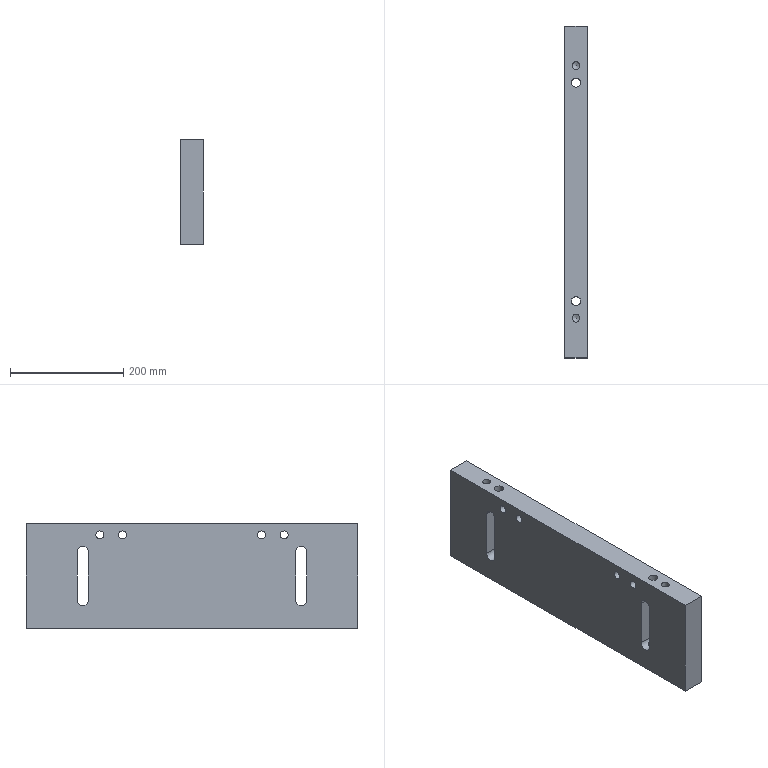Part | STEP file | 1 solid | 32 faces | box 40 x 585 x 185 mm | volume 4078797 mm3 | cylinder 17 | plane 10 | cone 5 | commonest cylinder face diameters 14 x9 16 x4 20 x4
STEP:
#1=CARTESIAN_POINT('',(-360.,-182.5,-242.));
#2=VERTEX_POINT('',#1);
#3=CARTESIAN_POINT('',(-360.,-202.5,-242.));
#4=VERTEX_POINT('',#3);
#5=CARTESIAN_POINT('',(-360.,-192.5,-242.));
#6=DIRECTION('',(-1.,0.,0.));
#7=DIRECTION('',(0.,0.,1.));
#8=AXIS2_PLACEMENT_3D('',#5,#6,#7);
#9=CIRCLE('',#8,10.);
#10=EDGE_CURVE('',#2,#4,#9,.T.);
#11=ORIENTED_EDGE('',*,*,#10,.F.);
#12=CARTESIAN_POINT('',(-360.,-182.5,-157.));
#13=VERTEX_POINT('',#12);
#14=CARTESIAN_POINT('',(-360.,-182.5,-292.));
#15=DIRECTION('',(0.,0.,1.));
#16=VECTOR('',#15,1.);
#17=LINE('',#14,#16);
#18=EDGE_CURVE('',#2,#13,#17,.T.);
#19=ORIENTED_EDGE('',*,*,#18,.T.);
#20=CARTESIAN_POINT('',(-360.,-202.5,-157.));
#21=VERTEX_POINT('',#20);
#22=CARTESIAN_POINT('',(-360.,-192.5,-157.));
#23=DIRECTION('',(-1.,0.,0.));
#24=DIRECTION('',(0.,0.,1.));
#25=AXIS2_PLACEMENT_3D('',#22,#23,#24);
#26=CIRCLE('',#25,10.);
#27=EDGE_CURVE('',#21,#13,#26,.T.);
#28=ORIENTED_EDGE('',*,*,#27,.F.);
#29=CARTESIAN_POINT('',(-360.,-202.5,-107.));
#30=DIRECTION('',(0.,0.,1.));
#31=VECTOR('',#30,1.);
#32=LINE('',#29,#31);
#33=EDGE_CURVE('',#4,#21,#32,.T.);
#34=ORIENTED_EDGE('',*,*,#33,.F.);
#35=EDGE_LOOP('',(#11,#19,#28,#34));
#36=FACE_BOUND('',#35,.T.);
#37=CARTESIAN_POINT('',(-360.,-292.5,-292.));
#38=VERTEX_POINT('',#37);
#39=CARTESIAN_POINT('',(-360.,-292.5,-107.));
#40=VERTEX_POINT('',#39);
#41=CARTESIAN_POINT('',(-360.,-292.5,-107.));
#42=DIRECTION('',(0.,0.,1.));
#43=VECTOR('',#42,1.);
#44=LINE('',#41,#43);
#45=EDGE_CURVE('',#38,#40,#44,.T.);
#46=ORIENTED_EDGE('',*,*,#45,.T.);
#47=CARTESIAN_POINT('',(-360.,292.5,-107.));
#48=VERTEX_POINT('',#47);
#49=CARTESIAN_POINT('',(-360.,-1.,-107.));
#50=DIRECTION('',(0.,-1.,0.));
#51=VECTOR('',#50,1.);
#52=LINE('',#49,#51);
#53=EDGE_CURVE('',#48,#40,#52,.T.);
#54=ORIENTED_EDGE('',*,*,#53,.F.);
#55=CARTESIAN_POINT('',(-360.,292.5,-292.));
#56=VERTEX_POINT('',#55);
#57=CARTESIAN_POINT('',(-360.,292.5,-107.));
#58=DIRECTION('',(0.,0.,1.));
#59=VECTOR('',#58,1.);
#60=LINE('',#57,#59);
#61=EDGE_CURVE('',#56,#48,#60,.T.);
#62=ORIENTED_EDGE('',*,*,#61,.F.);
#63=CARTESIAN_POINT('',(-360.,-1.,-292.));
#64=DIRECTION('',(0.,-1.,0.));
#65=VECTOR('',#64,1.);
#66=LINE('',#63,#65);
#67=EDGE_CURVE('',#56,#38,#66,.T.);
#68=ORIENTED_EDGE('',*,*,#67,.T.);
#69=EDGE_LOOP('',(#46,#54,#62,#68));
#70=FACE_BOUND('',#69,.T.);
#71=CARTESIAN_POINT('',(-360.,-162.5,-120.));
#72=VERTEX_POINT('',#71);
#73=CARTESIAN_POINT('',(-360.,-162.5,-127.));
#74=DIRECTION('',(-1.,0.,0.));
#75=DIRECTION('',(0.,0.,1.));
#76=AXIS2_PLACEMENT_3D('',#73,#74,#75);
#77=CIRCLE('',#76,7.);
#78=EDGE_CURVE('',#72,#72,#77,.T.);
#79=ORIENTED_EDGE('',*,*,#78,.F.);
#80=EDGE_LOOP('',(#79));
#81=FACE_BOUND('',#80,.T.);
#82=CARTESIAN_POINT('',(-360.,-122.5,-120.));
#83=VERTEX_POINT('',#82);
#84=CARTESIAN_POINT('',(-360.,-122.5,-127.));
#85=DIRECTION('',(1.,0.,0.));
#86=DIRECTION('',(0.,0.,1.));
#87=AXIS2_PLACEMENT_3D('',#84,#85,#86);
#88=CIRCLE('',#87,7.);
#89=EDGE_CURVE('',#83,#83,#88,.T.);
#90=ORIENTED_EDGE('',*,*,#89,.T.);
#91=EDGE_LOOP('',(#90));
#92=FACE_BOUND('',#91,.T.);
#93=CARTESIAN_POINT('',(-360.,162.5,-120.));
#94=VERTEX_POINT('',#93);
#95=CARTESIAN_POINT('',(-360.,162.5,-127.));
#96=DIRECTION('',(1.,0.,0.));
#97=DIRECTION('',(0.,0.,1.));
#98=AXIS2_PLACEMENT_3D('',#95,#96,#97);
#99=CIRCLE('',#98,7.);
#100=EDGE_CURVE('',#94,#94,#99,.T.);
#101=ORIENTED_EDGE('',*,*,#100,.T.);
#102=EDGE_LOOP('',(#101));
#103=FACE_BOUND('',#102,.T.);
#104=CARTESIAN_POINT('',(-360.,122.5,-120.));
#105=VERTEX_POINT('',#104);
#106=CARTESIAN_POINT('',(-360.,122.5,-127.));
#107=DIRECTION('',(-1.,0.,0.));
#108=DIRECTION('',(0.,0.,1.));
#109=AXIS2_PLACEMENT_3D('',#106,#107,#108);
#110=CIRCLE('',#109,7.);
#111=EDGE_CURVE('',#105,#105,#110,.T.);
#112=ORIENTED_EDGE('',*,*,#111,.F.);
#113=EDGE_LOOP('',(#112));
#114=FACE_BOUND('',#113,.T.);
#115=CARTESIAN_POINT('',(-360.,202.5,-242.));
#116=VERTEX_POINT('',#115);
#117=CARTESIAN_POINT('',(-360.,182.5,-242.));
#118=VERTEX_POINT('',#117);
#119=CARTESIAN_POINT('',(-360.,192.5,-242.));
#120=DIRECTION('',(-1.,0.,0.));
#121=DIRECTION('',(0.,0.,1.));
#122=AXIS2_PLACEMENT_3D('',#119,#120,#121);
#123=CIRCLE('',#122,10.);
#124=EDGE_CURVE('',#116,#118,#123,.T.);
#125=ORIENTED_EDGE('',*,*,#124,.F.);
#126=CARTESIAN_POINT('',(-360.,202.5,-157.));
#127=VERTEX_POINT('',#126);
#128=CARTESIAN_POINT('',(-360.,202.5,-292.));
#129=DIRECTION('',(0.,0.,1.));
#130=VECTOR('',#129,1.);
#131=LINE('',#128,#130);
#132=EDGE_CURVE('',#116,#127,#131,.T.);
#133=ORIENTED_EDGE('',*,*,#132,.T.);
#134=CARTESIAN_POINT('',(-360.,182.5,-157.));
#135=VERTEX_POINT('',#134);
#136=CARTESIAN_POINT('',(-360.,192.5,-157.));
#137=DIRECTION('',(-1.,0.,0.));
#138=DIRECTION('',(0.,0.,1.));
#139=AXIS2_PLACEMENT_3D('',#136,#137,#138);
#140=CIRCLE('',#139,10.);
#141=EDGE_CURVE('',#135,#127,#140,.T.);
#142=ORIENTED_EDGE('',*,*,#141,.F.);
#143=CARTESIAN_POINT('',(-360.,182.5,-107.));
#144=DIRECTION('',(0.,0.,1.));
#145=VECTOR('',#144,1.);
#146=LINE('',#143,#145);
#147=EDGE_CURVE('',#118,#135,#146,.T.);
#148=ORIENTED_EDGE('',*,*,#147,.F.);
#149=EDGE_LOOP('',(#125,#133,#142,#148));
#150=FACE_BOUND('',#149,.T.);
#151=CARTESIAN_POINT('',(-360.,-1.,-107.));
#152=DIRECTION('',(-1.,0.,0.));
#153=DIRECTION('',(0.,-1.,0.));
#154=AXIS2_PLACEMENT_3D('',#151,#152,#153);
#155=PLANE('',#154);
#156=ADVANCED_FACE('',(#36,#70,#81,#92,#103,#114,#150),#155,.T.);
#157=CARTESIAN_POINT('',(-320.,-202.5,-242.));
#158=VERTEX_POINT('',#157);
#159=CARTESIAN_POINT('',(-320.,-182.5,-242.));
#160=VERTEX_POINT('',#159);
#161=CARTESIAN_POINT('',(-320.,-192.5,-242.));
#162=DIRECTION('',(1.,0.,0.));
#163=DIRECTION('',(0.,0.,-1.));
#164=AXIS2_PLACEMENT_3D('',#161,#162,#163);
#165=CIRCLE('',#164,10.);
#166=EDGE_CURVE('',#158,#160,#165,.T.);
#167=ORIENTED_EDGE('',*,*,#166,.F.);
#168=CARTESIAN_POINT('',(-320.,-202.5,-157.));
#169=VERTEX_POINT('',#168);
#170=CARTESIAN_POINT('',(-320.,-202.5,-292.));
#171=DIRECTION('',(0.,0.,1.));
#172=VECTOR('',#171,1.);
#173=LINE('',#170,#172);
#174=EDGE_CURVE('',#158,#169,#173,.T.);
#175=ORIENTED_EDGE('',*,*,#174,.T.);
#176=CARTESIAN_POINT('',(-320.,-182.5,-157.));
#177=VERTEX_POINT('',#176);
#178=CARTESIAN_POINT('',(-320.,-192.5,-157.));
#179=DIRECTION('',(1.,0.,0.));
#180=DIRECTION('',(0.,0.,-1.));
#181=AXIS2_PLACEMENT_3D('',#178,#179,#180);
#182=CIRCLE('',#181,10.);
#183=EDGE_CURVE('',#177,#169,#182,.T.);
#184=ORIENTED_EDGE('',*,*,#183,.F.);
#185=CARTESIAN_POINT('',(-320.,-182.5,-107.));
#186=DIRECTION('',(0.,0.,1.));
#187=VECTOR('',#186,1.);
#188=LINE('',#185,#187);
#189=EDGE_CURVE('',#160,#177,#188,.T.);
#190=ORIENTED_EDGE('',*,*,#189,.F.);
#191=EDGE_LOOP('',(#167,#175,#184,#190));
#192=FACE_BOUND('',#191,.T.);
#193=CARTESIAN_POINT('',(-320.,122.5,-134.));
#194=VERTEX_POINT('',#193);
#195=CARTESIAN_POINT('',(-320.,122.5,-127.));
#196=DIRECTION('',(-1.,0.,0.));
#197=DIRECTION('',(0.,0.,-1.));
#198=AXIS2_PLACEMENT_3D('',#195,#196,#197);
#199=CIRCLE('',#198,7.);
#200=EDGE_CURVE('',#194,#194,#199,.T.);
#201=ORIENTED_EDGE('',*,*,#200,.T.);
#202=EDGE_LOOP('',(#201));
#203=FACE_BOUND('',#202,.T.);
#204=CARTESIAN_POINT('',(-320.,162.5,-134.));
#205=VERTEX_POINT('',#204);
#206=CARTESIAN_POINT('',(-320.,162.5,-127.));
#207=DIRECTION('',(1.,0.,0.));
#208=DIRECTION('',(0.,0.,-1.));
#209=AXIS2_PLACEMENT_3D('',#206,#207,#208);
#210=CIRCLE('',#209,7.);
#211=EDGE_CURVE('',#205,#205,#210,.T.);
#212=ORIENTED_EDGE('',*,*,#211,.F.);
#213=EDGE_LOOP('',(#212));
#214=FACE_BOUND('',#213,.T.);
#215=CARTESIAN_POINT('',(-320.,-122.5,-134.));
#216=VERTEX_POINT('',#215);
#217=CARTESIAN_POINT('',(-320.,-122.5,-127.));
#218=DIRECTION('',(1.,0.,0.));
#219=DIRECTION('',(0.,0.,-1.));
#220=AXIS2_PLACEMENT_3D('',#217,#218,#219);
#221=CIRCLE('',#220,7.);
#222=EDGE_CURVE('',#216,#216,#221,.T.);
#223=ORIENTED_EDGE('',*,*,#222,.F.);
#224=EDGE_LOOP('',(#223));
#225=FACE_BOUND('',#224,.T.);
#226=CARTESIAN_POINT('',(-320.,-162.5,-134.));
#227=VERTEX_POINT('',#226);
#228=CARTESIAN_POINT('',(-320.,-162.5,-127.));
#229=DIRECTION('',(-1.,0.,0.));
#230=DIRECTION('',(0.,0.,-1.));
#231=AXIS2_PLACEMENT_3D('',#228,#229,#230);
#232=CIRCLE('',#231,7.);
#233=EDGE_CURVE('',#227,#227,#232,.T.);
#234=ORIENTED_EDGE('',*,*,#233,.T.);
#235=EDGE_LOOP('',(#234));
#236=FACE_BOUND('',#235,.T.);
#237=CARTESIAN_POINT('',(-320.,292.5,-292.));
#238=VERTEX_POINT('',#237);
#239=CARTESIAN_POINT('',(-320.,292.5,-107.));
#240=VERTEX_POINT('',#239);
#241=CARTESIAN_POINT('',(-320.,292.5,-107.));
#242=DIRECTION('',(0.,0.,1.));
#243=VECTOR('',#242,1.);
#244=LINE('',#241,#243);
#245=EDGE_CURVE('',#238,#240,#244,.T.);
#246=ORIENTED_EDGE('',*,*,#245,.T.);
#247=CARTESIAN_POINT('',(-320.,-292.5,-107.));
#248=VERTEX_POINT('',#247);
#249=CARTESIAN_POINT('',(-320.,-1.,-107.));
#250=DIRECTION('',(0.,1.,0.));
#251=VECTOR('',#250,1.);
#252=LINE('',#249,#251);
#253=EDGE_CURVE('',#248,#240,#252,.T.);
#254=ORIENTED_EDGE('',*,*,#253,.F.);
#255=CARTESIAN_POINT('',(-320.,-292.5,-292.));
#256=VERTEX_POINT('',#255);
#257=CARTESIAN_POINT('',(-320.,-292.5,-107.));
#258=DIRECTION('',(0.,0.,1.));
#259=VECTOR('',#258,1.);
#260=LINE('',#257,#259);
#261=EDGE_CURVE('',#256,#248,#260,.T.);
#262=ORIENTED_EDGE('',*,*,#261,.F.);
#263=CARTESIAN_POINT('',(-320.,-1.,-292.));
#264=DIRECTION('',(0.,1.,0.));
#265=VECTOR('',#264,1.);
#266=LINE('',#263,#265);
#267=EDGE_CURVE('',#256,#238,#266,.T.);
#268=ORIENTED_EDGE('',*,*,#267,.T.);
#269=EDGE_LOOP('',(#246,#254,#262,#268));
#270=FACE_BOUND('',#269,.T.);
#271=CARTESIAN_POINT('',(-320.,182.5,-242.));
#272=VERTEX_POINT('',#271);
#273=CARTESIAN_POINT('',(-320.,202.5,-242.));
#274=VERTEX_POINT('',#273);
#275=CARTESIAN_POINT('',(-320.,192.5,-242.));
#276=DIRECTION('',(1.,0.,0.));
#277=DIRECTION('',(0.,0.,-1.));
#278=AXIS2_PLACEMENT_3D('',#275,#276,#277);
#279=CIRCLE('',#278,10.);
#280=EDGE_CURVE('',#272,#274,#279,.T.);
#281=ORIENTED_EDGE('',*,*,#280,.F.);
#282=CARTESIAN_POINT('',(-320.,182.5,-157.));
#283=VERTEX_POINT('',#282);
#284=CARTESIAN_POINT('',(-320.,182.5,-292.));
#285=DIRECTION('',(0.,0.,1.));
#286=VECTOR('',#285,1.);
#287=LINE('',#284,#286);
#288=EDGE_CURVE('',#272,#283,#287,.T.);
#289=ORIENTED_EDGE('',*,*,#288,.T.);
#290=CARTESIAN_POINT('',(-320.,202.5,-157.));
#291=VERTEX_POINT('',#290);
#292=CARTESIAN_POINT('',(-320.,192.5,-157.));
#293=DIRECTION('',(1.,0.,0.));
#294=DIRECTION('',(0.,0.,-1.));
#295=AXIS2_PLACEMENT_3D('',#292,#293,#294);
#296=CIRCLE('',#295,10.);
#297=EDGE_CURVE('',#291,#283,#296,.T.);
#298=ORIENTED_EDGE('',*,*,#297,.F.);
#299=CARTESIAN_POINT('',(-320.,202.5,-107.));
#300=DIRECTION('',(0.,0.,1.));
#301=VECTOR('',#300,1.);
#302=LINE('',#299,#301);
#303=EDGE_CURVE('',#274,#291,#302,.T.);
#304=ORIENTED_EDGE('',*,*,#303,.F.);
#305=EDGE_LOOP('',(#281,#289,#298,#304));
#306=FACE_BOUND('',#305,.T.);
#307=CARTESIAN_POINT('',(-320.,-1.,-107.));
#308=DIRECTION('',(1.,0.,0.));
#309=DIRECTION('',(0.,1.,0.));
#310=AXIS2_PLACEMENT_3D('',#307,#308,#309);
#311=PLANE('',#310);
#312=ADVANCED_FACE('',(#192,#203,#214,#225,#236,#270,#306),#311,.T.);
#313=ORIENTED_EDGE('',*,*,#61,.T.);
#314=CARTESIAN_POINT('',(98.5,292.5,-107.));
#315=DIRECTION('',(-1.,0.,0.));
#316=VECTOR('',#315,1.);
#317=LINE('',#314,#316);
#318=EDGE_CURVE('',#240,#48,#317,.T.);
#319=ORIENTED_EDGE('',*,*,#318,.F.);
#320=ORIENTED_EDGE('',*,*,#245,.F.);
#321=CARTESIAN_POINT('',(98.5,292.5,-292.));
#322=DIRECTION('',(-1.,0.,0.));
#323=VECTOR('',#322,1.);
#324=LINE('',#321,#323);
#325=EDGE_CURVE('',#238,#56,#324,.T.);
#326=ORIENTED_EDGE('',*,*,#325,.T.);
#327=EDGE_LOOP('',(#313,#319,#320,#326));
#328=FACE_OUTER_BOUND('',#327,.T.);
#329=CARTESIAN_POINT('',(98.5,292.5,-107.));
#330=DIRECTION('',(0.,1.,0.));
#331=DIRECTION('',(-1.,0.,0.));
#332=AXIS2_PLACEMENT_3D('',#329,#330,#331);
#333=PLANE('',#332);
#334=ADVANCED_FACE('',(#328),#333,.T.);
#335=CARTESIAN_POINT('',(98.5,-292.5,-292.));
#336=DIRECTION('',(1.,0.,0.));
#337=VECTOR('',#336,1.);
#338=LINE('',#335,#337);
#339=EDGE_CURVE('',#38,#256,#338,.T.);
#340=ORIENTED_EDGE('',*,*,#339,.T.);
#341=ORIENTED_EDGE('',*,*,#261,.T.);
#342=CARTESIAN_POINT('',(98.5,-292.5,-107.));
#343=DIRECTION('',(1.,0.,0.));
#344=VECTOR('',#343,1.);
#345=LINE('',#342,#344);
#346=EDGE_CURVE('',#40,#248,#345,.T.);
#347=ORIENTED_EDGE('',*,*,#346,.F.);
#348=ORIENTED_EDGE('',*,*,#45,.F.);
#349=EDGE_LOOP('',(#340,#341,#347,#348));
#350=FACE_OUTER_BOUND('',#349,.T.);
#351=CARTESIAN_POINT('',(98.5,-292.5,-107.));
#352=DIRECTION('',(0.,-1.,0.));
#353=DIRECTION('',(1.,0.,0.));
#354=AXIS2_PLACEMENT_3D('',#351,#352,#353);
#355=PLANE('',#354);
#356=ADVANCED_FACE('',(#350),#355,.T.);
#357=CARTESIAN_POINT('',(-348.,192.5,-107.));
#358=VERTEX_POINT('',#357);
#359=CARTESIAN_POINT('',(-340.,192.5,-107.));
#360=DIRECTION('',(0.,0.,1.));
#361=DIRECTION('',(-1.,0.,0.));
#362=AXIS2_PLACEMENT_3D('',#359,#360,#361);
#363=CIRCLE('',#362,8.);
#364=EDGE_CURVE('',#358,#358,#363,.T.);
#365=ORIENTED_EDGE('',*,*,#364,.F.);
#366=EDGE_LOOP('',(#365));
#367=FACE_BOUND('',#366,.T.);
#368=CARTESIAN_POINT('',(-348.,-192.5,-107.));
#369=VERTEX_POINT('',#368);
#370=CARTESIAN_POINT('',(-340.,-192.5,-107.));
#371=DIRECTION('',(0.,0.,-1.));
#372=DIRECTION('',(-1.,0.,0.));
#373=AXIS2_PLACEMENT_3D('',#370,#371,#372);
#374=CIRCLE('',#373,8.);
#375=EDGE_CURVE('',#369,#369,#374,.T.);
#376=ORIENTED_EDGE('',*,*,#375,.T.);
#377=EDGE_LOOP('',(#376));
#378=FACE_BOUND('',#377,.T.);
#379=ORIENTED_EDGE('',*,*,#253,.T.);
#380=ORIENTED_EDGE('',*,*,#318,.T.);
#381=ORIENTED_EDGE('',*,*,#53,.T.);
#382=ORIENTED_EDGE('',*,*,#346,.T.);
#383=EDGE_LOOP('',(#379,#380,#381,#382));
#384=FACE_BOUND('',#383,.T.);
#385=CARTESIAN_POINT('',(-347.,-222.5,-107.));
#386=VERTEX_POINT('',#385);
#387=CARTESIAN_POINT('',(-340.,-222.5,-107.));
#388=DIRECTION('',(0.,0.,-1.));
#389=DIRECTION('',(-1.,0.,0.));
#390=AXIS2_PLACEMENT_3D('',#387,#388,#389);
#391=CIRCLE('',#390,7.);
#392=EDGE_CURVE('',#386,#386,#391,.T.);
#393=ORIENTED_EDGE('',*,*,#392,.T.);
#394=EDGE_LOOP('',(#393));
#395=FACE_BOUND('',#394,.T.);
#396=CARTESIAN_POINT('',(-347.,222.5,-107.));
#397=VERTEX_POINT('',#396);
#398=CARTESIAN_POINT('',(-340.,222.5,-107.));
#399=DIRECTION('',(0.,0.,1.));
#400=DIRECTION('',(-1.,0.,0.));
#401=AXIS2_PLACEMENT_3D('',#398,#399,#400);
#402=CIRCLE('',#401,7.);
#403=EDGE_CURVE('',#397,#397,#402,.T.);
#404=ORIENTED_EDGE('',*,*,#403,.F.);
#405=EDGE_LOOP('',(#404));
#406=FACE_BOUND('',#405,.T.);
#407=CARTESIAN_POINT('',(98.5,-1.,-107.));
#408=DIRECTION('',(0.,0.,1.));
#409=DIRECTION('',(1.,0.,0.));
#410=AXIS2_PLACEMENT_3D('',#407,#408,#409);
#411=PLANE('',#410);
#412=ADVANCED_FACE('',(#367,#378,#384,#395,#406),#411,.T.);
#413=CARTESIAN_POINT('',(-332.,-192.5,-292.));
#414=VERTEX_POINT('',#413);
#415=CARTESIAN_POINT('',(-340.,-192.5,-292.));
#416=DIRECTION('',(0.,0.,-1.));
#417=DIRECTION('',(1.,0.,0.));
#418=AXIS2_PLACEMENT_3D('',#415,#416,#417);
#419=CIRCLE('',#418,8.);
#420=EDGE_CURVE('',#414,#414,#419,.T.);
#421=ORIENTED_EDGE('',*,*,#420,.F.);
#422=EDGE_LOOP('',(#421));
#423=FACE_BOUND('',#422,.T.);
#424=CARTESIAN_POINT('',(-332.,192.5,-292.));
#425=VERTEX_POINT('',#424);
#426=CARTESIAN_POINT('',(-340.,192.5,-292.));
#427=DIRECTION('',(0.,0.,1.));
#428=DIRECTION('',(1.,0.,0.));
#429=AXIS2_PLACEMENT_3D('',#426,#427,#428);
#430=CIRCLE('',#429,8.);
#431=EDGE_CURVE('',#425,#425,#430,.T.);
#432=ORIENTED_EDGE('',*,*,#431,.T.);
#433=EDGE_LOOP('',(#432));
#434=FACE_BOUND('',#433,.T.);
#435=ORIENTED_EDGE('',*,*,#267,.F.);
#436=ORIENTED_EDGE('',*,*,#339,.F.);
#437=ORIENTED_EDGE('',*,*,#67,.F.);
#438=ORIENTED_EDGE('',*,*,#325,.F.);
#439=EDGE_LOOP('',(#435,#436,#437,#438));
#440=FACE_BOUND('',#439,.T.);
#441=CARTESIAN_POINT('',(-333.,267.5,-292.));
#442=VERTEX_POINT('',#441);
#443=CARTESIAN_POINT('',(-340.,267.5,-292.));
#444=DIRECTION('',(0.,0.,1.));
#445=DIRECTION('',(1.,0.,0.));
#446=AXIS2_PLACEMENT_3D('',#443,#444,#445);
#447=CIRCLE('',#446,7.);
#448=EDGE_CURVE('',#442,#442,#447,.T.);
#449=ORIENTED_EDGE('',*,*,#448,.T.);
#450=EDGE_LOOP('',(#449));
#451=FACE_BOUND('',#450,.T.);
#452=CARTESIAN_POINT('',(-333.,-267.5,-292.));
#453=VERTEX_POINT('',#452);
#454=CARTESIAN_POINT('',(-340.,-267.5,-292.));
#455=DIRECTION('',(0.,0.,-1.));
#456=DIRECTION('',(1.,0.,0.));
#457=AXIS2_PLACEMENT_3D('',#454,#455,#456);
#458=CIRCLE('',#457,7.);
#459=EDGE_CURVE('',#453,#453,#458,.T.);
#460=ORIENTED_EDGE('',*,*,#459,.F.);
#461=EDGE_LOOP('',(#460));
#462=FACE_BOUND('',#461,.T.);
#463=CARTESIAN_POINT('',(-333.,0.,-292.));
#464=VERTEX_POINT('',#463);
#465=CARTESIAN_POINT('',(-340.,0.,-292.));
#466=DIRECTION('',(0.,0.,1.));
#467=DIRECTION('',(1.,0.,0.));
#468=AXIS2_PLACEMENT_3D('',#465,#466,#467);
#469=CIRCLE('',#468,7.);
#470=EDGE_CURVE('',#464,#464,#469,.T.);
#471=ORIENTED_EDGE('',*,*,#470,.T.);
#472=EDGE_LOOP('',(#471));
#473=FACE_BOUND('',#472,.T.);
#474=CARTESIAN_POINT('',(88.5,-1.,-292.));
#475=DIRECTION('',(0.,0.,-1.));
#476=DIRECTION('',(1.,0.,0.));
#477=AXIS2_PLACEMENT_3D('',#474,#475,#476);
#478=PLANE('',#477);
#479=ADVANCED_FACE('',(#423,#434,#440,#451,#462,#473),#478,.T.);
#480=CARTESIAN_POINT('',(-333.,-222.5,-147.));
#481=VERTEX_POINT('',#480);
#482=CARTESIAN_POINT('',(-340.,-222.5,-147.));
#483=DIRECTION('',(0.,0.,1.));
#484=DIRECTION('',(1.,0.,0.));
#485=AXIS2_PLACEMENT_3D('',#482,#483,#484);
#486=CIRCLE('',#485,7.);
#487=EDGE_CURVE('',#481,#481,#486,.T.);
#488=ORIENTED_EDGE('',*,*,#487,.F.);
#489=EDGE_LOOP('',(#488));
#490=FACE_BOUND('',#489,.T.);
#491=ORIENTED_EDGE('',*,*,#392,.F.);
#492=EDGE_LOOP('',(#491));
#493=FACE_BOUND('',#492,.T.);
#494=CARTESIAN_POINT('',(-340.,-222.5,-107.));
#495=DIRECTION('',(0.,0.,-1.));
#496=DIRECTION('',(1.,0.,0.));
#497=AXIS2_PLACEMENT_3D('',#494,#495,#496);
#498=CYLINDRICAL_SURFACE('',#497,7.);
#499=ADVANCED_FACE('',(#490,#493),#498,.F.);
#500=ORIENTED_EDGE('',*,*,#487,.T.);
#501=EDGE_LOOP('',(#500));
#502=FACE_BOUND('',#501,.T.);
#503=CARTESIAN_POINT('',(-340.,-222.5,-150.));
#504=VERTEX_POINT('',#503);
#505=VERTEX_LOOP('',#504);
#506=FACE_BOUND('',#505,.T.);
#507=CARTESIAN_POINT('',(-340.,-222.5,-150.));
#508=DIRECTION('',(0.,0.,1.));
#509=DIRECTION('',(1.,0.,0.));
#510=AXIS2_PLACEMENT_3D('',#507,#508,#509);
#511=CONICAL_SURFACE('',#510,0.,66.801);
#512=ADVANCED_FACE('',(#502,#506),#511,.F.);
#513=CARTESIAN_POINT('',(-333.,222.5,-147.));
#514=VERTEX_POINT('',#513);
#515=CARTESIAN_POINT('',(-340.,222.5,-147.));
#516=DIRECTION('',(0.,0.,-1.));
#517=DIRECTION('',(1.,0.,0.));
#518=AXIS2_PLACEMENT_3D('',#515,#516,#517);
#519=CIRCLE('',#518,7.);
#520=EDGE_CURVE('',#514,#514,#519,.T.);
#521=ORIENTED_EDGE('',*,*,#520,.T.);
#522=EDGE_LOOP('',(#521));
#523=FACE_BOUND('',#522,.T.);
#524=ORIENTED_EDGE('',*,*,#403,.T.);
#525=EDGE_LOOP('',(#524));
#526=FACE_BOUND('',#525,.T.);
#527=CARTESIAN_POINT('',(-340.,222.5,-107.));
#528=DIRECTION('',(0.,0.,-1.));
#529=DIRECTION('',(1.,0.,0.));
#530=AXIS2_PLACEMENT_3D('',#527,#528,#529);
#531=CYLINDRICAL_SURFACE('',#530,7.);
#532=ADVANCED_FACE('',(#523,#526),#531,.F.);
#533=ORIENTED_EDGE('',*,*,#520,.F.);
#534=EDGE_LOOP('',(#533));
#535=FACE_BOUND('',#534,.T.);
#536=CARTESIAN_POINT('',(-340.,222.5,-150.));
#537=VERTEX_POINT('',#536);
#538=VERTEX_LOOP('',#537);
#539=FACE_BOUND('',#538,.T.);
#540=CARTESIAN_POINT('',(-340.,222.5,-150.));
#541=DIRECTION('',(0.,0.,1.));
#542=DIRECTION('',(1.,0.,0.));
#543=AXIS2_PLACEMENT_3D('',#540,#541,#542);
#544=CONICAL_SURFACE('',#543,0.,66.801);
#545=ADVANCED_FACE('',(#535,#539),#544,.F.);
#546=CARTESIAN_POINT('',(-347.,267.5,-252.));
#547=VERTEX_POINT('',#546);
#548=CARTESIAN_POINT('',(-340.,267.5,-252.));
#549=DIRECTION('',(0.,0.,-1.));
#550=DIRECTION('',(-1.,0.,0.));
#551=AXIS2_PLACEMENT_3D('',#548,#549,#550);
#552=CIRCLE('',#551,7.);
#553=EDGE_CURVE('',#547,#547,#552,.T.);
#554=ORIENTED_EDGE('',*,*,#553,.F.);
#555=EDGE_LOOP('',(#554));
#556=FACE_BOUND('',#555,.T.);
#557=ORIENTED_EDGE('',*,*,#448,.F.);
#558=EDGE_LOOP('',(#557));
#559=FACE_BOUND('',#558,.T.);
#560=CARTESIAN_POINT('',(-340.,267.5,-292.));
#561=DIRECTION('',(0.,0.,1.));
#562=DIRECTION('',(-1.,0.,0.));
#563=AXIS2_PLACEMENT_3D('',#560,#561,#562);
#564=CYLINDRICAL_SURFACE('',#563,7.);
#565=ADVANCED_FACE('',(#556,#559),#564,.F.);
#566=ORIENTED_EDGE('',*,*,#553,.T.);
#567=EDGE_LOOP('',(#566));
#568=FACE_BOUND('',#567,.T.);
#569=CARTESIAN_POINT('',(-340.,267.5,-249.));
#570=VERTEX_POINT('',#569);
#571=VERTEX_LOOP('',#570);
#572=FACE_BOUND('',#571,.T.);
#573=CARTESIAN_POINT('',(-340.,267.5,-249.));
#574=DIRECTION('',(0.,0.,-1.));
#575=DIRECTION('',(-1.,0.,0.));
#576=AXIS2_PLACEMENT_3D('',#573,#574,#575);
#577=CONICAL_SURFACE('',#576,0.,66.801);
#578=ADVANCED_FACE('',(#568,#572),#577,.F.);
#579=CARTESIAN_POINT('',(-347.,-267.5,-252.));
#580=VERTEX_POINT('',#579);
#581=CARTESIAN_POINT('',(-340.,-267.5,-252.));
#582=DIRECTION('',(0.,0.,1.));
#583=DIRECTION('',(-1.,0.,0.));
#584=AXIS2_PLACEMENT_3D('',#581,#582,#583);
#585=CIRCLE('',#584,7.);
#586=EDGE_CURVE('',#580,#580,#585,.T.);
#587=ORIENTED_EDGE('',*,*,#586,.T.);
#588=EDGE_LOOP('',(#587));
#589=FACE_BOUND('',#588,.T.);
#590=ORIENTED_EDGE('',*,*,#459,.T.);
#591=EDGE_LOOP('',(#590));
#592=FACE_BOUND('',#591,.T.);
#593=CARTESIAN_POINT('',(-340.,-267.5,-292.));
#594=DIRECTION('',(0.,0.,1.));
#595=DIRECTION('',(-1.,0.,0.));
#596=AXIS2_PLACEMENT_3D('',#593,#594,#595);
#597=CYLINDRICAL_SURFACE('',#596,7.);
#598=ADVANCED_FACE('',(#589,#592),#597,.F.);
#599=ORIENTED_EDGE('',*,*,#586,.F.);
#600=EDGE_LOOP('',(#599));
#601=FACE_BOUND('',#600,.T.);
#602=CARTESIAN_POINT('',(-340.,-267.5,-249.));
#603=VERTEX_POINT('',#602);
#604=VERTEX_LOOP('',#603);
#605=FACE_BOUND('',#604,.T.);
#606=CARTESIAN_POINT('',(-340.,-267.5,-249.));
#607=DIRECTION('',(0.,0.,-1.));
#608=DIRECTION('',(-1.,0.,0.));
#609=AXIS2_PLACEMENT_3D('',#606,#607,#608);
#610=CONICAL_SURFACE('',#609,0.,66.801);
#611=ADVANCED_FACE('',(#601,#605),#610,.F.);
#612=CARTESIAN_POINT('',(-347.,0.,-252.));
#613=VERTEX_POINT('',#612);
#614=CARTESIAN_POINT('',(-340.,0.,-252.));
#615=DIRECTION('',(0.,0.,-1.));
#616=DIRECTION('',(-1.,0.,0.));
#617=AXIS2_PLACEMENT_3D('',#614,#615,#616);
#618=CIRCLE('',#617,7.);
#619=EDGE_CURVE('',#613,#613,#618,.T.);
#620=ORIENTED_EDGE('',*,*,#619,.F.);
#621=EDGE_LOOP('',(#620));
#622=FACE_BOUND('',#621,.T.);
#623=ORIENTED_EDGE('',*,*,#470,.F.);
#624=EDGE_LOOP('',(#623));
#625=FACE_BOUND('',#624,.T.);
#626=CARTESIAN_POINT('',(-340.,0.,-292.));
#627=DIRECTION('',(0.,0.,1.));
#628=DIRECTION('',(-1.,0.,0.));
#629=AXIS2_PLACEMENT_3D('',#626,#627,#628);
#630=CYLINDRICAL_SURFACE('',#629,7.);
#631=ADVANCED_FACE('',(#622,#625),#630,.F.);
#632=ORIENTED_EDGE('',*,*,#619,.T.);
#633=EDGE_LOOP('',(#632));
#634=FACE_BOUND('',#633,.T.);
#635=CARTESIAN_POINT('',(-340.,0.,-249.));
#636=VERTEX_POINT('',#635);
#637=VERTEX_LOOP('',#636);
#638=FACE_BOUND('',#637,.T.);
#639=CARTESIAN_POINT('',(-340.,0.,-249.));
#640=DIRECTION('',(0.,0.,-1.));
#641=DIRECTION('',(-1.,0.,0.));
#642=AXIS2_PLACEMENT_3D('',#639,#640,#641);
#643=CONICAL_SURFACE('',#642,0.,66.801);
#644=ADVANCED_FACE('',(#634,#638),#643,.F.);
#645=ORIENTED_EDGE('',*,*,#233,.F.);
#646=EDGE_LOOP('',(#645));
#647=FACE_BOUND('',#646,.T.);
#648=ORIENTED_EDGE('',*,*,#78,.T.);
#649=EDGE_LOOP('',(#648));
#650=FACE_BOUND('',#649,.T.);
#651=CARTESIAN_POINT('',(-360.,-162.5,-127.));
#652=DIRECTION('',(1.,0.,0.));
#653=DIRECTION('',(0.,0.,-1.));
#654=AXIS2_PLACEMENT_3D('',#651,#652,#653);
#655=CYLINDRICAL_SURFACE('',#654,7.);
#656=ADVANCED_FACE('',(#647,#650),#655,.F.);
#657=ORIENTED_EDGE('',*,*,#222,.T.);
#658=EDGE_LOOP('',(#657));
#659=FACE_BOUND('',#658,.T.);
#660=ORIENTED_EDGE('',*,*,#89,.F.);
#661=EDGE_LOOP('',(#660));
#662=FACE_BOUND('',#661,.T.);
#663=CARTESIAN_POINT('',(-360.,-122.5,-127.));
#664=DIRECTION('',(1.,0.,0.));
#665=DIRECTION('',(0.,0.,-1.));
#666=AXIS2_PLACEMENT_3D('',#663,#664,#665);
#667=CYLINDRICAL_SURFACE('',#666,7.);
#668=ADVANCED_FACE('',(#659,#662),#667,.F.);
#669=ORIENTED_EDGE('',*,*,#211,.T.);
#670=EDGE_LOOP('',(#669));
#671=FACE_BOUND('',#670,.T.);
#672=ORIENTED_EDGE('',*,*,#100,.F.);
#673=EDGE_LOOP('',(#672));
#674=FACE_BOUND('',#673,.T.);
#675=CARTESIAN_POINT('',(-360.,162.5,-127.));
#676=DIRECTION('',(1.,0.,0.));
#677=DIRECTION('',(0.,0.,-1.));
#678=AXIS2_PLACEMENT_3D('',#675,#676,#677);
#679=CYLINDRICAL_SURFACE('',#678,7.);
#680=ADVANCED_FACE('',(#671,#674),#679,.F.);
#681=ORIENTED_EDGE('',*,*,#200,.F.);
#682=EDGE_LOOP('',(#681));
#683=FACE_BOUND('',#682,.T.);
#684=ORIENTED_EDGE('',*,*,#111,.T.);
#685=EDGE_LOOP('',(#684));
#686=FACE_BOUND('',#685,.T.);
#687=CARTESIAN_POINT('',(-360.,122.5,-127.));
#688=DIRECTION('',(1.,0.,0.));
#689=DIRECTION('',(0.,0.,-1.));
#690=AXIS2_PLACEMENT_3D('',#687,#688,#689);
#691=CYLINDRICAL_SURFACE('',#690,7.);
#692=ADVANCED_FACE('',(#683,#686),#691,.F.);
#693=CARTESIAN_POINT('',(-348.,-192.5,-147.));
#694=VERTEX_POINT('',#693);
#695=CARTESIAN_POINT('',(-348.,-193.621,-147.));
#696=CARTESIAN_POINT('',(-348.,-190.259,-147.));
#697=CARTESIAN_POINT('',(-347.029,-188.195,-147.816));
#698=CARTESIAN_POINT('',(-344.91,-186.107,-149.264));
#699=CARTESIAN_POINT('',(-344.084,-185.547,-149.789));
#700=CARTESIAN_POINT('',(-342.219,-184.747,-150.656));
#701=CARTESIAN_POINT('',(-341.125,-184.503,-150.996));
#702=CARTESIAN_POINT('',(-338.914,-184.497,-151.004));
#703=CARTESIAN_POINT('',(-337.834,-184.731,-150.676));
#704=CARTESIAN_POINT('',(-335.939,-185.531,-149.804));
#705=CARTESIAN_POINT('',(-335.124,-186.079,-149.286));
#706=CARTESIAN_POINT('',(-333.694,-187.477,-148.311));
#707=CARTESIAN_POINT('',(-333.105,-188.307,-147.864));
#708=CARTESIAN_POINT('',(-332.249,-190.253,-147.202));
#709=CARTESIAN_POINT('',(-332.006,-191.354,-147.005));
#710=CARTESIAN_POINT('',(-331.994,-193.56,-146.995));
#711=CARTESIAN_POINT('',(-332.227,-194.671,-147.184));
#712=CARTESIAN_POINT('',(-333.067,-196.632,-147.835));
#713=CARTESIAN_POINT('',(-333.662,-197.483,-148.288));
#714=CARTESIAN_POINT('',(-335.078,-198.885,-149.256));
#715=CARTESIAN_POINT('',(-335.907,-199.448,-149.783));
#716=CARTESIAN_POINT('',(-337.766,-200.248,-150.65));
#717=CARTESIAN_POINT('',(-338.855,-200.496,-150.995));
#718=CARTESIAN_POINT('',(-341.089,-200.504,-151.005));
#719=CARTESIAN_POINT('',(-342.169,-200.268,-150.675));
#720=CARTESIAN_POINT('',(-344.06,-199.469,-149.804));
#721=CARTESIAN_POINT('',(-344.881,-198.917,-149.283));
#722=CARTESIAN_POINT('',(-346.314,-197.514,-148.306));
#723=CARTESIAN_POINT('',(-346.902,-196.683,-147.858));
#724=CARTESIAN_POINT('',(-347.757,-194.729,-147.197));
#725=CARTESIAN_POINT('',(-348.,-193.621,-147.));
#726=CARTESIAN_POINT('',(-348.,-190.259,-147.));
#727=B_SPLINE_CURVE_WITH_KNOTS('',3,(#695,#696,#697,#698,#699,#700,#701,#702,#703,#704,#705,#706,#707,#708,#709,#710,#711,#712,#713,#714,#715,#716,#717,#718,#719,#720,#721,#722,#723,#724,#725,#726),.UNSPECIFIED.,.T.,.F.,(2,2,2,2,2,2,2,2,2,2,2,2,2,2,2,2,2,2),(-0.0625,0.,0.125,0.1875,0.25,0.3125,0.375,0.4375,0.5,0.5625,0.625,0.6875,0.75,0.8125,0.875,0.9375,1.,1.125),.UNSPECIFIED.);
#728=EDGE_CURVE('',#694,#694,#727,.T.);
#729=ORIENTED_EDGE('',*,*,#728,.T.);
#730=EDGE_LOOP('',(#729));
#731=FACE_BOUND('',#730,.T.);
#732=ORIENTED_EDGE('',*,*,#375,.F.);
#733=EDGE_LOOP('',(#732));
#734=FACE_BOUND('',#733,.T.);
#735=CARTESIAN_POINT('',(-340.,-192.5,-107.));
#736=DIRECTION('',(0.,0.,-1.));
#737=DIRECTION('',(-1.,0.,0.));
#738=AXIS2_PLACEMENT_3D('',#735,#736,#737);
#739=CYLINDRICAL_SURFACE('',#738,8.);
#740=ADVANCED_FACE('',(#731,#734),#739,.F.);
#741=CARTESIAN_POINT('',(-348.,192.5,-147.));
#742=VERTEX_POINT('',#741);
#743=CARTESIAN_POINT('',(-348.,191.379,-147.));
#744=CARTESIAN_POINT('',(-348.,194.741,-147.));
#745=CARTESIAN_POINT('',(-347.029,196.805,-147.816));
#746=CARTESIAN_POINT('',(-344.91,198.893,-149.264));
#747=CARTESIAN_POINT('',(-344.084,199.453,-149.789));
#748=CARTESIAN_POINT('',(-342.219,200.253,-150.656));
#749=CARTESIAN_POINT('',(-341.125,200.497,-150.996));
#750=CARTESIAN_POINT('',(-338.914,200.503,-151.004));
#751=CARTESIAN_POINT('',(-337.834,200.269,-150.676));
#752=CARTESIAN_POINT('',(-335.939,199.469,-149.804));
#753=CARTESIAN_POINT('',(-335.124,198.921,-149.286));
#754=CARTESIAN_POINT('',(-333.694,197.523,-148.311));
#755=CARTESIAN_POINT('',(-333.105,196.693,-147.864));
#756=CARTESIAN_POINT('',(-332.249,194.747,-147.202));
#757=CARTESIAN_POINT('',(-332.006,193.646,-147.005));
#758=CARTESIAN_POINT('',(-331.994,191.44,-146.995));
#759=CARTESIAN_POINT('',(-332.227,190.329,-147.184));
#760=CARTESIAN_POINT('',(-333.067,188.368,-147.835));
#761=CARTESIAN_POINT('',(-333.662,187.517,-148.288));
#762=CARTESIAN_POINT('',(-335.078,186.115,-149.256));
#763=CARTESIAN_POINT('',(-335.907,185.552,-149.783));
#764=CARTESIAN_POINT('',(-337.766,184.752,-150.65));
#765=CARTESIAN_POINT('',(-338.855,184.504,-150.995));
#766=CARTESIAN_POINT('',(-341.089,184.496,-151.005));
#767=CARTESIAN_POINT('',(-342.169,184.732,-150.675));
#768=CARTESIAN_POINT('',(-344.06,185.531,-149.804));
#769=CARTESIAN_POINT('',(-344.881,186.083,-149.283));
#770=CARTESIAN_POINT('',(-346.314,187.486,-148.306));
#771=CARTESIAN_POINT('',(-346.902,188.317,-147.858));
#772=CARTESIAN_POINT('',(-347.757,190.271,-147.197));
#773=CARTESIAN_POINT('',(-348.,191.379,-147.));
#774=CARTESIAN_POINT('',(-348.,194.741,-147.));
#775=B_SPLINE_CURVE_WITH_KNOTS('',3,(#743,#744,#745,#746,#747,#748,#749,#750,#751,#752,#753,#754,#755,#756,#757,#758,#759,#760,#761,#762,#763,#764,#765,#766,#767,#768,#769,#770,#771,#772,#773,#774),.UNSPECIFIED.,.T.,.F.,(2,2,2,2,2,2,2,2,2,2,2,2,2,2,2,2,2,2),(-0.0625,0.,0.125,0.1875,0.25,0.3125,0.375,0.4375,0.5,0.5625,0.625,0.6875,0.75,0.8125,0.875,0.9375,1.,1.125),.UNSPECIFIED.);
#776=EDGE_CURVE('',#742,#742,#775,.T.);
#777=ORIENTED_EDGE('',*,*,#776,.T.);
#778=EDGE_LOOP('',(#777));
#779=FACE_BOUND('',#778,.T.);
#780=ORIENTED_EDGE('',*,*,#364,.T.);
#781=EDGE_LOOP('',(#780));
#782=FACE_BOUND('',#781,.T.);
#783=CARTESIAN_POINT('',(-340.,192.5,-107.));
#784=DIRECTION('',(0.,0.,-1.));
#785=DIRECTION('',(-1.,0.,0.));
#786=AXIS2_PLACEMENT_3D('',#783,#784,#785);
#787=CYLINDRICAL_SURFACE('',#786,8.);
#788=ADVANCED_FACE('',(#779,#782),#787,.F.);
#789=CARTESIAN_POINT('',(-332.,192.5,-252.));
#790=VERTEX_POINT('',#789);
#791=CARTESIAN_POINT('',(-332.,191.379,-252.));
#792=CARTESIAN_POINT('',(-332.,194.741,-252.));
#793=CARTESIAN_POINT('',(-332.971,196.805,-251.184));
#794=CARTESIAN_POINT('',(-335.09,198.893,-249.736));
#795=CARTESIAN_POINT('',(-335.916,199.453,-249.211));
#796=CARTESIAN_POINT('',(-337.781,200.253,-248.344));
#797=CARTESIAN_POINT('',(-338.875,200.497,-248.004));
#798=CARTESIAN_POINT('',(-341.086,200.503,-247.996));
#799=CARTESIAN_POINT('',(-342.166,200.269,-248.324));
#800=CARTESIAN_POINT('',(-344.061,199.469,-249.196));
#801=CARTESIAN_POINT('',(-344.876,198.921,-249.714));
#802=CARTESIAN_POINT('',(-346.306,197.523,-250.689));
#803=CARTESIAN_POINT('',(-346.895,196.693,-251.136));
#804=CARTESIAN_POINT('',(-347.751,194.747,-251.798));
#805=CARTESIAN_POINT('',(-347.994,193.646,-251.995));
#806=CARTESIAN_POINT('',(-348.006,191.44,-252.005));
#807=CARTESIAN_POINT('',(-347.773,190.329,-251.816));
#808=CARTESIAN_POINT('',(-346.933,188.368,-251.165));
#809=CARTESIAN_POINT('',(-346.338,187.517,-250.712));
#810=CARTESIAN_POINT('',(-344.922,186.115,-249.744));
#811=CARTESIAN_POINT('',(-344.093,185.552,-249.217));
#812=CARTESIAN_POINT('',(-342.234,184.752,-248.35));
#813=CARTESIAN_POINT('',(-341.145,184.504,-248.005));
#814=CARTESIAN_POINT('',(-338.911,184.496,-247.995));
#815=CARTESIAN_POINT('',(-337.831,184.732,-248.325));
#816=CARTESIAN_POINT('',(-335.94,185.531,-249.196));
#817=CARTESIAN_POINT('',(-335.119,186.083,-249.717));
#818=CARTESIAN_POINT('',(-333.686,187.486,-250.694));
#819=CARTESIAN_POINT('',(-333.098,188.317,-251.142));
#820=CARTESIAN_POINT('',(-332.243,190.271,-251.803));
#821=CARTESIAN_POINT('',(-332.,191.379,-252.));
#822=CARTESIAN_POINT('',(-332.,194.741,-252.));
#823=B_SPLINE_CURVE_WITH_KNOTS('',3,(#791,#792,#793,#794,#795,#796,#797,#798,#799,#800,#801,#802,#803,#804,#805,#806,#807,#808,#809,#810,#811,#812,#813,#814,#815,#816,#817,#818,#819,#820,#821,#822),.UNSPECIFIED.,.T.,.F.,(2,2,2,2,2,2,2,2,2,2,2,2,2,2,2,2,2,2),(-0.0625,0.,0.125,0.1875,0.25,0.3125,0.375,0.4375,0.5,0.5625,0.625,0.6875,0.75,0.8125,0.875,0.9375,1.,1.125),.UNSPECIFIED.);
#824=EDGE_CURVE('',#790,#790,#823,.T.);
#825=ORIENTED_EDGE('',*,*,#824,.T.);
#826=EDGE_LOOP('',(#825));
#827=FACE_BOUND('',#826,.T.);
#828=ORIENTED_EDGE('',*,*,#431,.F.);
#829=EDGE_LOOP('',(#828));
#830=FACE_BOUND('',#829,.T.);
#831=CARTESIAN_POINT('',(-340.,192.5,-292.));
#832=DIRECTION('',(0.,0.,1.));
#833=DIRECTION('',(1.,0.,0.));
#834=AXIS2_PLACEMENT_3D('',#831,#832,#833);
#835=CYLINDRICAL_SURFACE('',#834,8.);
#836=ADVANCED_FACE('',(#827,#830),#835,.F.);
#837=CARTESIAN_POINT('',(-332.,-192.5,-252.));
#838=VERTEX_POINT('',#837);
#839=CARTESIAN_POINT('',(-332.,-193.621,-252.));
#840=CARTESIAN_POINT('',(-332.,-190.259,-252.));
#841=CARTESIAN_POINT('',(-332.971,-188.195,-251.184));
#842=CARTESIAN_POINT('',(-335.09,-186.107,-249.736));
#843=CARTESIAN_POINT('',(-335.916,-185.547,-249.211));
#844=CARTESIAN_POINT('',(-337.781,-184.747,-248.344));
#845=CARTESIAN_POINT('',(-338.875,-184.503,-248.004));
#846=CARTESIAN_POINT('',(-341.086,-184.497,-247.996));
#847=CARTESIAN_POINT('',(-342.166,-184.731,-248.324));
#848=CARTESIAN_POINT('',(-344.061,-185.531,-249.196));
#849=CARTESIAN_POINT('',(-344.876,-186.079,-249.714));
#850=CARTESIAN_POINT('',(-346.306,-187.477,-250.689));
#851=CARTESIAN_POINT('',(-346.895,-188.307,-251.136));
#852=CARTESIAN_POINT('',(-347.751,-190.253,-251.798));
#853=CARTESIAN_POINT('',(-347.994,-191.354,-251.995));
#854=CARTESIAN_POINT('',(-348.006,-193.56,-252.005));
#855=CARTESIAN_POINT('',(-347.773,-194.671,-251.816));
#856=CARTESIAN_POINT('',(-346.933,-196.632,-251.165));
#857=CARTESIAN_POINT('',(-346.338,-197.483,-250.712));
#858=CARTESIAN_POINT('',(-344.922,-198.885,-249.744));
#859=CARTESIAN_POINT('',(-344.093,-199.448,-249.217));
#860=CARTESIAN_POINT('',(-342.234,-200.248,-248.35));
#861=CARTESIAN_POINT('',(-341.145,-200.496,-248.005));
#862=CARTESIAN_POINT('',(-338.911,-200.504,-247.995));
#863=CARTESIAN_POINT('',(-337.831,-200.268,-248.325));
#864=CARTESIAN_POINT('',(-335.94,-199.469,-249.196));
#865=CARTESIAN_POINT('',(-335.119,-198.917,-249.717));
#866=CARTESIAN_POINT('',(-333.686,-197.514,-250.694));
#867=CARTESIAN_POINT('',(-333.098,-196.683,-251.142));
#868=CARTESIAN_POINT('',(-332.243,-194.729,-251.803));
#869=CARTESIAN_POINT('',(-332.,-193.621,-252.));
#870=CARTESIAN_POINT('',(-332.,-190.259,-252.));
#871=B_SPLINE_CURVE_WITH_KNOTS('',3,(#839,#840,#841,#842,#843,#844,#845,#846,#847,#848,#849,#850,#851,#852,#853,#854,#855,#856,#857,#858,#859,#860,#861,#862,#863,#864,#865,#866,#867,#868,#869,#870),.UNSPECIFIED.,.T.,.F.,(2,2,2,2,2,2,2,2,2,2,2,2,2,2,2,2,2,2),(-0.0625,0.,0.125,0.1875,0.25,0.3125,0.375,0.4375,0.5,0.5625,0.625,0.6875,0.75,0.8125,0.875,0.9375,1.,1.125),.UNSPECIFIED.);
#872=EDGE_CURVE('',#838,#838,#871,.T.);
#873=ORIENTED_EDGE('',*,*,#872,.T.);
#874=EDGE_LOOP('',(#873));
#875=FACE_BOUND('',#874,.T.);
#876=ORIENTED_EDGE('',*,*,#420,.T.);
#877=EDGE_LOOP('',(#876));
#878=FACE_BOUND('',#877,.T.);
#879=CARTESIAN_POINT('',(-340.,-192.5,-292.));
#880=DIRECTION('',(0.,0.,1.));
#881=DIRECTION('',(1.,0.,0.));
#882=AXIS2_PLACEMENT_3D('',#879,#880,#881);
#883=CYLINDRICAL_SURFACE('',#882,8.);
#884=ADVANCED_FACE('',(#875,#878),#883,.F.);
#885=ORIENTED_EDGE('',*,*,#183,.T.);
#886=CARTESIAN_POINT('',(-340.,-202.5,-157.));
#887=DIRECTION('',(1.,0.,0.));
#888=VECTOR('',#887,1.);
#889=LINE('',#886,#888);
#890=EDGE_CURVE('',#21,#169,#889,.T.);
#891=ORIENTED_EDGE('',*,*,#890,.F.);
#892=ORIENTED_EDGE('',*,*,#27,.T.);
#893=CARTESIAN_POINT('',(-340.,-182.5,-157.));
#894=DIRECTION('',(-1.,0.,0.));
#895=VECTOR('',#894,1.);
#896=LINE('',#893,#895);
#897=EDGE_CURVE('',#177,#13,#896,.T.);
#898=ORIENTED_EDGE('',*,*,#897,.F.);
#899=EDGE_LOOP('',(#885,#891,#892,#898));
#900=FACE_BOUND('',#899,.T.);
#901=ORIENTED_EDGE('',*,*,#728,.F.);
#902=EDGE_LOOP('',(#901));
#903=FACE_BOUND('',#902,.T.);
#904=CARTESIAN_POINT('',(-340.,-192.5,-157.));
#905=DIRECTION('',(-1.,0.,0.));
#906=DIRECTION('',(0.,0.,1.));
#907=AXIS2_PLACEMENT_3D('',#904,#905,#906);
#908=CYLINDRICAL_SURFACE('',#907,10.);
#909=ADVANCED_FACE('',(#900,#903),#908,.F.);
#910=ORIENTED_EDGE('',*,*,#10,.T.);
#911=CARTESIAN_POINT('',(-340.,-202.5,-242.));
#912=DIRECTION('',(-1.,0.,0.));
#913=VECTOR('',#912,1.);
#914=LINE('',#911,#913);
#915=EDGE_CURVE('',#158,#4,#914,.T.);
#916=ORIENTED_EDGE('',*,*,#915,.F.);
#917=ORIENTED_EDGE('',*,*,#166,.T.);
#918=CARTESIAN_POINT('',(-340.,-182.5,-242.));
#919=DIRECTION('',(1.,0.,0.));
#920=VECTOR('',#919,1.);
#921=LINE('',#918,#920);
#922=EDGE_CURVE('',#2,#160,#921,.T.);
#923=ORIENTED_EDGE('',*,*,#922,.F.);
#924=EDGE_LOOP('',(#910,#916,#917,#923));
#925=FACE_BOUND('',#924,.T.);
#926=ORIENTED_EDGE('',*,*,#872,.F.);
#927=EDGE_LOOP('',(#926));
#928=FACE_BOUND('',#927,.T.);
#929=CARTESIAN_POINT('',(-340.,-192.5,-242.));
#930=DIRECTION('',(1.,0.,0.));
#931=DIRECTION('',(0.,0.,-1.));
#932=AXIS2_PLACEMENT_3D('',#929,#930,#931);
#933=CYLINDRICAL_SURFACE('',#932,10.);
#934=ADVANCED_FACE('',(#925,#928),#933,.F.);
#935=ORIENTED_EDGE('',*,*,#33,.T.);
#936=ORIENTED_EDGE('',*,*,#890,.T.);
#937=ORIENTED_EDGE('',*,*,#174,.F.);
#938=ORIENTED_EDGE('',*,*,#915,.T.);
#939=EDGE_LOOP('',(#935,#936,#937,#938));
#940=FACE_OUTER_BOUND('',#939,.T.);
#941=CARTESIAN_POINT('',(-340.,-202.5,-292.));
#942=DIRECTION('',(0.,-1.,0.));
#943=DIRECTION('',(0.,0.,1.));
#944=AXIS2_PLACEMENT_3D('',#941,#942,#943);
#945=PLANE('',#944);
#946=ADVANCED_FACE('',(#940),#945,.F.);
#947=ORIENTED_EDGE('',*,*,#189,.T.);
#948=ORIENTED_EDGE('',*,*,#897,.T.);
#949=ORIENTED_EDGE('',*,*,#18,.F.);
#950=ORIENTED_EDGE('',*,*,#922,.T.);
#951=EDGE_LOOP('',(#947,#948,#949,#950));
#952=FACE_OUTER_BOUND('',#951,.T.);
#953=CARTESIAN_POINT('',(-340.,-182.5,-292.));
#954=DIRECTION('',(0.,1.,0.));
#955=DIRECTION('',(0.,0.,-1.));
#956=AXIS2_PLACEMENT_3D('',#953,#954,#955);
#957=PLANE('',#956);
#958=ADVANCED_FACE('',(#952),#957,.F.);
#959=ORIENTED_EDGE('',*,*,#297,.T.);
#960=CARTESIAN_POINT('',(-340.,182.5,-157.));
#961=DIRECTION('',(1.,0.,0.));
#962=VECTOR('',#961,1.);
#963=LINE('',#960,#962);
#964=EDGE_CURVE('',#135,#283,#963,.T.);
#965=ORIENTED_EDGE('',*,*,#964,.F.);
#966=ORIENTED_EDGE('',*,*,#141,.T.);
#967=CARTESIAN_POINT('',(-340.,202.5,-157.));
#968=DIRECTION('',(-1.,0.,0.));
#969=VECTOR('',#968,1.);
#970=LINE('',#967,#969);
#971=EDGE_CURVE('',#291,#127,#970,.T.);
#972=ORIENTED_EDGE('',*,*,#971,.F.);
#973=EDGE_LOOP('',(#959,#965,#966,#972));
#974=FACE_BOUND('',#973,.T.);
#975=ORIENTED_EDGE('',*,*,#776,.F.);
#976=EDGE_LOOP('',(#975));
#977=FACE_BOUND('',#976,.T.);
#978=CARTESIAN_POINT('',(-340.,192.5,-157.));
#979=DIRECTION('',(-1.,0.,0.));
#980=DIRECTION('',(0.,0.,1.));
#981=AXIS2_PLACEMENT_3D('',#978,#979,#980);
#982=CYLINDRICAL_SURFACE('',#981,10.);
#983=ADVANCED_FACE('',(#974,#977),#982,.F.);
#984=ORIENTED_EDGE('',*,*,#124,.T.);
#985=CARTESIAN_POINT('',(-340.,182.5,-242.));
#986=DIRECTION('',(-1.,0.,0.));
#987=VECTOR('',#986,1.);
#988=LINE('',#985,#987);
#989=EDGE_CURVE('',#272,#118,#988,.T.);
#990=ORIENTED_EDGE('',*,*,#989,.F.);
#991=ORIENTED_EDGE('',*,*,#280,.T.);
#992=CARTESIAN_POINT('',(-340.,202.5,-242.));
#993=DIRECTION('',(1.,0.,0.));
#994=VECTOR('',#993,1.);
#995=LINE('',#992,#994);
#996=EDGE_CURVE('',#116,#274,#995,.T.);
#997=ORIENTED_EDGE('',*,*,#996,.F.);
#998=EDGE_LOOP('',(#984,#990,#991,#997));
#999=FACE_BOUND('',#998,.T.);
#1000=ORIENTED_EDGE('',*,*,#824,.F.);
#1001=EDGE_LOOP('',(#1000));
#1002=FACE_BOUND('',#1001,.T.);
#1003=CARTESIAN_POINT('',(-340.,192.5,-242.));
#1004=DIRECTION('',(1.,0.,0.));
#1005=DIRECTION('',(0.,0.,-1.));
#1006=AXIS2_PLACEMENT_3D('',#1003,#1004,#1005);
#1007=CYLINDRICAL_SURFACE('',#1006,10.);
#1008=ADVANCED_FACE('',(#999,#1002),#1007,.F.);
#1009=ORIENTED_EDGE('',*,*,#147,.T.);
#1010=ORIENTED_EDGE('',*,*,#964,.T.);
#1011=ORIENTED_EDGE('',*,*,#288,.F.);
#1012=ORIENTED_EDGE('',*,*,#989,.T.);
#1013=EDGE_LOOP('',(#1009,#1010,#1011,#1012));
#1014=FACE_OUTER_BOUND('',#1013,.T.);
#1015=CARTESIAN_POINT('',(-340.,182.5,-292.));
#1016=DIRECTION('',(0.,-1.,0.));
#1017=DIRECTION('',(0.,0.,1.));
#1018=AXIS2_PLACEMENT_3D('',#1015,#1016,#1017);
#1019=PLANE('',#1018);
#1020=ADVANCED_FACE('',(#1014),#1019,.F.);
#1021=ORIENTED_EDGE('',*,*,#303,.T.);
#1022=ORIENTED_EDGE('',*,*,#971,.T.);
#1023=ORIENTED_EDGE('',*,*,#132,.F.);
#1024=ORIENTED_EDGE('',*,*,#996,.T.);
#1025=EDGE_LOOP('',(#1021,#1022,#1023,#1024));
#1026=FACE_OUTER_BOUND('',#1025,.T.);
#1027=CARTESIAN_POINT('',(-340.,202.5,-292.));
#1028=DIRECTION('',(0.,1.,0.));
#1029=DIRECTION('',(0.,0.,-1.));
#1030=AXIS2_PLACEMENT_3D('',#1027,#1028,#1029);
#1031=PLANE('',#1030);
#1032=ADVANCED_FACE('',(#1026),#1031,.F.);
#1033=CLOSED_SHELL('',(#156,#312,#334,#356,#412,#479,#499,#512,#532,#545,#565,#578,#598,#611,#631,#644,#656,#668,#680,#692,#740,#788,#836,#884,#909,#934,#946,#958,#983,#1008,#1020,#1032));
#1034=MANIFOLD_SOLID_BREP('',#1033);
#1035=(LENGTH_UNIT()NAMED_UNIT(*)SI_UNIT(.MILLI.,.METRE.));
#1036=UNCERTAINTY_MEASURE_WITH_UNIT(LENGTH_MEASURE(0.0508),#1035,'','');
#1037=(NAMED_UNIT(*)PLANE_ANGLE_UNIT()SI_UNIT($,.RADIAN.));
#1038=PLANE_ANGLE_MEASURE_WITH_UNIT(PLANE_ANGLE_MEASURE(0.01745),#1037);
#1039=DIMENSIONAL_EXPONENTS(0.,0.,0.,0.,0.,0.,0.);
#1040=(CONVERSION_BASED_UNIT('DEGREE',#1038)NAMED_UNIT(#1039)PLANE_ANGLE_UNIT());
#1041=(NAMED_UNIT(*)SI_UNIT($,.STERADIAN.)SOLID_ANGLE_UNIT());
#1042=(GEOMETRIC_REPRESENTATION_CONTEXT(3)GLOBAL_UNCERTAINTY_ASSIGNED_CONTEXT((#1036))GLOBAL_UNIT_ASSIGNED_CONTEXT((#1035,#1040,#1041))REPRESENTATION_CONTEXT('',''));
#1043=ADVANCED_BREP_SHAPE_REPRESENTATION('',(#1034),#1042);